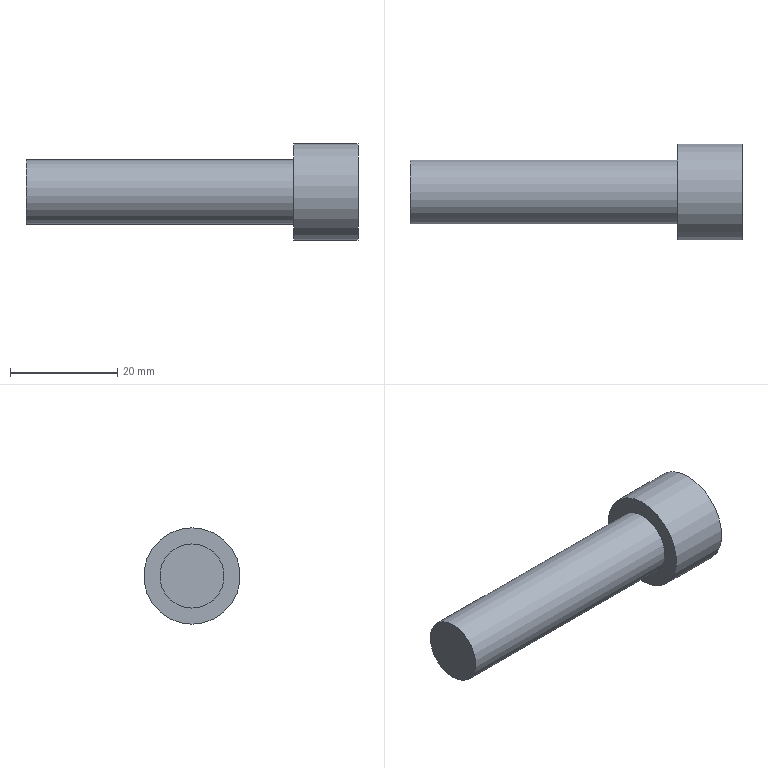Part | STEP file | lll_id6_x_t | 1 solid | 12 faces | box 62 x 18 x 18 mm | volume 8023 mm3 | plane 10 | cylinder 2 | commonest cylinder face diameters 12 x1 18 x1
STEP:
#1=CARTESIAN_POINT('',(169.,-73.,-48.5));
#2=VERTEX_POINT('',#1);
#3=CARTESIAN_POINT('',(169.,-73.,-39.5));
#4=DIRECTION('',(1.,0.,0.));
#5=DIRECTION('',(0.,0.,-1.));
#6=AXIS2_PLACEMENT_3D('',#3,#4,#5);
#7=CIRCLE('',#6,9.);
#8=EDGE_CURVE('',#2,#2,#7,.T.);
#9=ORIENTED_EDGE('',*,*,#8,.T.);
#10=EDGE_LOOP('',(#9));
#11=FACE_BOUND('',#10,.T.);
#12=CARTESIAN_POINT('',(169.,-68.,-36.613));
#13=VERTEX_POINT('',#12);
#14=CARTESIAN_POINT('',(169.,-68.,-42.387));
#15=VERTEX_POINT('',#14);
#16=CARTESIAN_POINT('',(169.,-68.,-36.613));
#17=DIRECTION('',(0.,0.,-1.));
#18=VECTOR('',#17,1.);
#19=LINE('',#16,#18);
#20=EDGE_CURVE('',#13,#15,#19,.T.);
#21=ORIENTED_EDGE('',*,*,#20,.T.);
#22=CARTESIAN_POINT('',(169.,-73.,-45.274));
#23=VERTEX_POINT('',#22);
#24=CARTESIAN_POINT('',(169.,-68.,-42.387));
#25=DIRECTION('',(0.,-0.866,-0.5));
#26=VECTOR('',#25,1.);
#27=LINE('',#24,#26);
#28=EDGE_CURVE('',#15,#23,#27,.T.);
#29=ORIENTED_EDGE('',*,*,#28,.T.);
#30=CARTESIAN_POINT('',(169.,-78.,-42.387));
#31=VERTEX_POINT('',#30);
#32=CARTESIAN_POINT('',(169.,-73.,-45.274));
#33=DIRECTION('',(0.,-0.866,0.5));
#34=VECTOR('',#33,1.);
#35=LINE('',#32,#34);
#36=EDGE_CURVE('',#23,#31,#35,.T.);
#37=ORIENTED_EDGE('',*,*,#36,.T.);
#38=CARTESIAN_POINT('',(169.,-78.,-36.613));
#39=VERTEX_POINT('',#38);
#40=CARTESIAN_POINT('',(169.,-78.,-42.387));
#41=DIRECTION('',(0.,0.,1.));
#42=VECTOR('',#41,1.);
#43=LINE('',#40,#42);
#44=EDGE_CURVE('',#31,#39,#43,.T.);
#45=ORIENTED_EDGE('',*,*,#44,.T.);
#46=CARTESIAN_POINT('',(169.,-73.,-33.726));
#47=VERTEX_POINT('',#46);
#48=CARTESIAN_POINT('',(169.,-78.,-36.613));
#49=DIRECTION('',(0.,0.866,0.5));
#50=VECTOR('',#49,1.);
#51=LINE('',#48,#50);
#52=EDGE_CURVE('',#39,#47,#51,.T.);
#53=ORIENTED_EDGE('',*,*,#52,.T.);
#54=CARTESIAN_POINT('',(169.,-73.,-33.726));
#55=DIRECTION('',(0.,0.866,-0.5));
#56=VECTOR('',#55,1.);
#57=LINE('',#54,#56);
#58=EDGE_CURVE('',#47,#13,#57,.T.);
#59=ORIENTED_EDGE('',*,*,#58,.T.);
#60=EDGE_LOOP('',(#21,#29,#37,#45,#53,#59));
#61=FACE_BOUND('',#60,.T.);
#62=CARTESIAN_POINT('',(169.,-73.,-48.5));
#63=DIRECTION('',(-1.,0.,0.));
#64=DIRECTION('',(0.,0.,1.));
#65=AXIS2_PLACEMENT_3D('',#62,#63,#64);
#66=PLANE('',#65);
#67=ADVANCED_FACE('',(#11,#61),#66,.F.);
#68=ORIENTED_EDGE('',*,*,#8,.F.);
#69=EDGE_LOOP('',(#68));
#70=FACE_BOUND('',#69,.T.);
#71=CARTESIAN_POINT('',(157.,-73.,-48.5));
#72=VERTEX_POINT('',#71);
#73=CARTESIAN_POINT('',(157.,-73.,-39.5));
#74=DIRECTION('',(1.,0.,0.));
#75=DIRECTION('',(0.,0.,-1.));
#76=AXIS2_PLACEMENT_3D('',#73,#74,#75);
#77=CIRCLE('',#76,9.);
#78=EDGE_CURVE('',#72,#72,#77,.T.);
#79=ORIENTED_EDGE('',*,*,#78,.T.);
#80=EDGE_LOOP('',(#79));
#81=FACE_BOUND('',#80,.T.);
#82=CARTESIAN_POINT('',(126.1,-73.,-39.5));
#83=DIRECTION('',(1.,0.,0.));
#84=DIRECTION('',(0.,0.,-1.));
#85=AXIS2_PLACEMENT_3D('',#82,#83,#84);
#86=CYLINDRICAL_SURFACE('',#85,9.);
#87=ADVANCED_FACE('',(#70,#81),#86,.T.);
#88=ORIENTED_EDGE('',*,*,#78,.F.);
#89=EDGE_LOOP('',(#88));
#90=FACE_BOUND('',#89,.T.);
#91=CARTESIAN_POINT('',(157.,-73.,-45.5));
#92=VERTEX_POINT('',#91);
#93=CARTESIAN_POINT('',(157.,-73.,-39.5));
#94=DIRECTION('',(1.,0.,0.));
#95=DIRECTION('',(0.,0.,-1.));
#96=AXIS2_PLACEMENT_3D('',#93,#94,#95);
#97=CIRCLE('',#96,6.);
#98=EDGE_CURVE('',#92,#92,#97,.T.);
#99=ORIENTED_EDGE('',*,*,#98,.T.);
#100=EDGE_LOOP('',(#99));
#101=FACE_BOUND('',#100,.T.);
#102=CARTESIAN_POINT('',(157.,-73.,-45.5));
#103=DIRECTION('',(1.,0.,0.));
#104=DIRECTION('',(0.,0.,-1.));
#105=AXIS2_PLACEMENT_3D('',#102,#103,#104);
#106=PLANE('',#105);
#107=ADVANCED_FACE('',(#90,#101),#106,.F.);
#108=ORIENTED_EDGE('',*,*,#98,.F.);
#109=EDGE_LOOP('',(#108));
#110=FACE_BOUND('',#109,.T.);
#111=CARTESIAN_POINT('',(107.,-73.,-45.5));
#112=VERTEX_POINT('',#111);
#113=CARTESIAN_POINT('',(107.,-73.,-39.5));
#114=DIRECTION('',(1.,0.,0.));
#115=DIRECTION('',(0.,0.,-1.));
#116=AXIS2_PLACEMENT_3D('',#113,#114,#115);
#117=CIRCLE('',#116,6.);
#118=EDGE_CURVE('',#112,#112,#117,.T.);
#119=ORIENTED_EDGE('',*,*,#118,.T.);
#120=EDGE_LOOP('',(#119));
#121=FACE_BOUND('',#120,.T.);
#122=CARTESIAN_POINT('',(126.1,-73.,-39.5));
#123=DIRECTION('',(1.,0.,0.));
#124=DIRECTION('',(0.,0.,-1.));
#125=AXIS2_PLACEMENT_3D('',#122,#123,#124);
#126=CYLINDRICAL_SURFACE('',#125,6.);
#127=ADVANCED_FACE('',(#110,#121),#126,.T.);
#128=ORIENTED_EDGE('',*,*,#118,.F.);
#129=EDGE_LOOP('',(#128));
#130=FACE_OUTER_BOUND('',#129,.T.);
#131=CARTESIAN_POINT('',(107.,-73.,-39.5));
#132=DIRECTION('',(1.,0.,0.));
#133=DIRECTION('',(0.,0.,-1.));
#134=AXIS2_PLACEMENT_3D('',#131,#132,#133);
#135=PLANE('',#134);
#136=ADVANCED_FACE('',(#130),#135,.F.);
#137=ORIENTED_EDGE('',*,*,#20,.F.);
#138=CARTESIAN_POINT('',(161.08,-68.,-36.613));
#139=VERTEX_POINT('',#138);
#140=CARTESIAN_POINT('',(161.08,-68.,-36.613));
#141=DIRECTION('',(-1.,0.,0.));
#142=VECTOR('',#141,1.);
#143=LINE('',#140,#142);
#144=EDGE_CURVE('',#13,#139,#143,.T.);
#145=ORIENTED_EDGE('',*,*,#144,.T.);
#146=CARTESIAN_POINT('',(161.08,-68.,-42.387));
#147=VERTEX_POINT('',#146);
#148=CARTESIAN_POINT('',(161.08,-68.,-36.613));
#149=DIRECTION('',(0.,0.,1.));
#150=VECTOR('',#149,1.);
#151=LINE('',#148,#150);
#152=EDGE_CURVE('',#147,#139,#151,.T.);
#153=ORIENTED_EDGE('',*,*,#152,.F.);
#154=CARTESIAN_POINT('',(161.08,-68.,-42.387));
#155=DIRECTION('',(-1.,0.,0.));
#156=VECTOR('',#155,1.);
#157=LINE('',#154,#156);
#158=EDGE_CURVE('',#15,#147,#157,.T.);
#159=ORIENTED_EDGE('',*,*,#158,.F.);
#160=EDGE_LOOP('',(#137,#145,#153,#159));
#161=FACE_OUTER_BOUND('',#160,.T.);
#162=CARTESIAN_POINT('',(161.08,-68.,-36.613));
#163=DIRECTION('',(0.,-1.,0.));
#164=DIRECTION('',(0.,0.,-1.));
#165=AXIS2_PLACEMENT_3D('',#162,#163,#164);
#166=PLANE('',#165);
#167=ADVANCED_FACE('',(#161),#166,.T.);
#168=ORIENTED_EDGE('',*,*,#28,.F.);
#169=ORIENTED_EDGE('',*,*,#158,.T.);
#170=CARTESIAN_POINT('',(161.08,-73.,-45.274));
#171=VERTEX_POINT('',#170);
#172=CARTESIAN_POINT('',(161.08,-68.,-42.387));
#173=DIRECTION('',(0.,0.866,0.5));
#174=VECTOR('',#173,1.);
#175=LINE('',#172,#174);
#176=EDGE_CURVE('',#171,#147,#175,.T.);
#177=ORIENTED_EDGE('',*,*,#176,.F.);
#178=CARTESIAN_POINT('',(161.08,-73.,-45.274));
#179=DIRECTION('',(-1.,0.,0.));
#180=VECTOR('',#179,1.);
#181=LINE('',#178,#180);
#182=EDGE_CURVE('',#23,#171,#181,.T.);
#183=ORIENTED_EDGE('',*,*,#182,.F.);
#184=EDGE_LOOP('',(#168,#169,#177,#183));
#185=FACE_OUTER_BOUND('',#184,.T.);
#186=CARTESIAN_POINT('',(161.08,-68.,-42.387));
#187=DIRECTION('',(0.,-0.5,0.866));
#188=DIRECTION('',(0.,-0.866,-0.5));
#189=AXIS2_PLACEMENT_3D('',#186,#187,#188);
#190=PLANE('',#189);
#191=ADVANCED_FACE('',(#185),#190,.T.);
#192=ORIENTED_EDGE('',*,*,#36,.F.);
#193=ORIENTED_EDGE('',*,*,#182,.T.);
#194=CARTESIAN_POINT('',(161.08,-78.,-42.387));
#195=VERTEX_POINT('',#194);
#196=CARTESIAN_POINT('',(161.08,-73.,-45.274));
#197=DIRECTION('',(0.,0.866,-0.5));
#198=VECTOR('',#197,1.);
#199=LINE('',#196,#198);
#200=EDGE_CURVE('',#195,#171,#199,.T.);
#201=ORIENTED_EDGE('',*,*,#200,.F.);
#202=CARTESIAN_POINT('',(161.08,-78.,-42.387));
#203=DIRECTION('',(-1.,0.,0.));
#204=VECTOR('',#203,1.);
#205=LINE('',#202,#204);
#206=EDGE_CURVE('',#31,#195,#205,.T.);
#207=ORIENTED_EDGE('',*,*,#206,.F.);
#208=EDGE_LOOP('',(#192,#193,#201,#207));
#209=FACE_OUTER_BOUND('',#208,.T.);
#210=CARTESIAN_POINT('',(161.08,-73.,-45.274));
#211=DIRECTION('',(0.,0.5,0.866));
#212=DIRECTION('',(0.,-0.866,0.5));
#213=AXIS2_PLACEMENT_3D('',#210,#211,#212);
#214=PLANE('',#213);
#215=ADVANCED_FACE('',(#209),#214,.T.);
#216=ORIENTED_EDGE('',*,*,#44,.F.);
#217=ORIENTED_EDGE('',*,*,#206,.T.);
#218=CARTESIAN_POINT('',(161.08,-78.,-36.613));
#219=VERTEX_POINT('',#218);
#220=CARTESIAN_POINT('',(161.08,-78.,-42.387));
#221=DIRECTION('',(0.,0.,-1.));
#222=VECTOR('',#221,1.);
#223=LINE('',#220,#222);
#224=EDGE_CURVE('',#219,#195,#223,.T.);
#225=ORIENTED_EDGE('',*,*,#224,.F.);
#226=CARTESIAN_POINT('',(161.08,-78.,-36.613));
#227=DIRECTION('',(-1.,0.,0.));
#228=VECTOR('',#227,1.);
#229=LINE('',#226,#228);
#230=EDGE_CURVE('',#39,#219,#229,.T.);
#231=ORIENTED_EDGE('',*,*,#230,.F.);
#232=EDGE_LOOP('',(#216,#217,#225,#231));
#233=FACE_OUTER_BOUND('',#232,.T.);
#234=CARTESIAN_POINT('',(161.08,-78.,-42.387));
#235=DIRECTION('',(0.,1.,0.));
#236=DIRECTION('',(0.,0.,1.));
#237=AXIS2_PLACEMENT_3D('',#234,#235,#236);
#238=PLANE('',#237);
#239=ADVANCED_FACE('',(#233),#238,.T.);
#240=ORIENTED_EDGE('',*,*,#52,.F.);
#241=ORIENTED_EDGE('',*,*,#230,.T.);
#242=CARTESIAN_POINT('',(161.08,-73.,-33.726));
#243=VERTEX_POINT('',#242);
#244=CARTESIAN_POINT('',(161.08,-78.,-36.613));
#245=DIRECTION('',(0.,-0.866,-0.5));
#246=VECTOR('',#245,1.);
#247=LINE('',#244,#246);
#248=EDGE_CURVE('',#243,#219,#247,.T.);
#249=ORIENTED_EDGE('',*,*,#248,.F.);
#250=CARTESIAN_POINT('',(161.08,-73.,-33.726));
#251=DIRECTION('',(-1.,0.,0.));
#252=VECTOR('',#251,1.);
#253=LINE('',#250,#252);
#254=EDGE_CURVE('',#47,#243,#253,.T.);
#255=ORIENTED_EDGE('',*,*,#254,.F.);
#256=EDGE_LOOP('',(#240,#241,#249,#255));
#257=FACE_OUTER_BOUND('',#256,.T.);
#258=CARTESIAN_POINT('',(161.08,-78.,-36.613));
#259=DIRECTION('',(0.,0.5,-0.866));
#260=DIRECTION('',(0.,0.866,0.5));
#261=AXIS2_PLACEMENT_3D('',#258,#259,#260);
#262=PLANE('',#261);
#263=ADVANCED_FACE('',(#257),#262,.T.);
#264=ORIENTED_EDGE('',*,*,#58,.F.);
#265=ORIENTED_EDGE('',*,*,#254,.T.);
#266=CARTESIAN_POINT('',(161.08,-73.,-33.726));
#267=DIRECTION('',(0.,-0.866,0.5));
#268=VECTOR('',#267,1.);
#269=LINE('',#266,#268);
#270=EDGE_CURVE('',#139,#243,#269,.T.);
#271=ORIENTED_EDGE('',*,*,#270,.F.);
#272=ORIENTED_EDGE('',*,*,#144,.F.);
#273=EDGE_LOOP('',(#264,#265,#271,#272));
#274=FACE_OUTER_BOUND('',#273,.T.);
#275=CARTESIAN_POINT('',(161.08,-73.,-33.726));
#276=DIRECTION('',(0.,-0.5,-0.866));
#277=DIRECTION('',(0.,0.866,-0.5));
#278=AXIS2_PLACEMENT_3D('',#275,#276,#277);
#279=PLANE('',#278);
#280=ADVANCED_FACE('',(#274),#279,.T.);
#281=ORIENTED_EDGE('',*,*,#152,.T.);
#282=ORIENTED_EDGE('',*,*,#270,.T.);
#283=ORIENTED_EDGE('',*,*,#248,.T.);
#284=ORIENTED_EDGE('',*,*,#224,.T.);
#285=ORIENTED_EDGE('',*,*,#200,.T.);
#286=ORIENTED_EDGE('',*,*,#176,.T.);
#287=EDGE_LOOP('',(#281,#282,#283,#284,#285,#286));
#288=FACE_OUTER_BOUND('',#287,.T.);
#289=CARTESIAN_POINT('',(161.08,-73.,-39.5));
#290=DIRECTION('',(-1.,0.,0.));
#291=DIRECTION('',(0.,0.,1.));
#292=AXIS2_PLACEMENT_3D('',#289,#290,#291);
#293=PLANE('',#292);
#294=ADVANCED_FACE('',(#288),#293,.F.);
#295=CLOSED_SHELL('',(#67,#87,#107,#127,#136,#167,#191,#215,#239,#263,#280,#294));
#296=MANIFOLD_SOLID_BREP('',#295);
#297=(LENGTH_UNIT()NAMED_UNIT(*)SI_UNIT(.MILLI.,.METRE.));
#298=UNCERTAINTY_MEASURE_WITH_UNIT(LENGTH_MEASURE(0.00002),#297,'','');
#299=(NAMED_UNIT(*)PLANE_ANGLE_UNIT()SI_UNIT($,.RADIAN.));
#300=PLANE_ANGLE_MEASURE_WITH_UNIT(PLANE_ANGLE_MEASURE(0.01745),#299);
#301=DIMENSIONAL_EXPONENTS(0.,0.,0.,0.,0.,0.,0.);
#302=(CONVERSION_BASED_UNIT('DEGREE',#300)NAMED_UNIT(#301)PLANE_ANGLE_UNIT());
#303=(NAMED_UNIT(*)SI_UNIT($,.STERADIAN.)SOLID_ANGLE_UNIT());
#304=(GEOMETRIC_REPRESENTATION_CONTEXT(3)GLOBAL_UNCERTAINTY_ASSIGNED_CONTEXT((#298))GLOBAL_UNIT_ASSIGNED_CONTEXT((#297,#302,#303))REPRESENTATION_CONTEXT('',''));
#305=ADVANCED_BREP_SHAPE_REPRESENTATION('',(#296),#304);